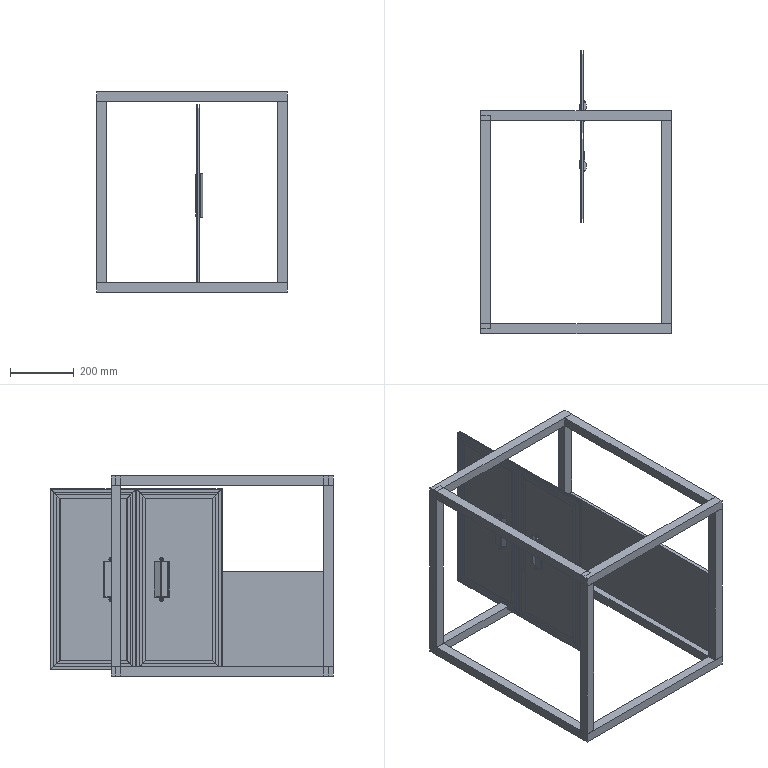Part | SolidWorks | 25 solids | 396 faces | box 600 x 890.825 x 630 mm | volume 10208073 mm3 | plane 284 | cylinder 88 | spline 8 | cone 8 | torus 8 | commonest cylinder face diameters 2 x44 4 x8 8 x8 10 x8 12 x8 52 x6